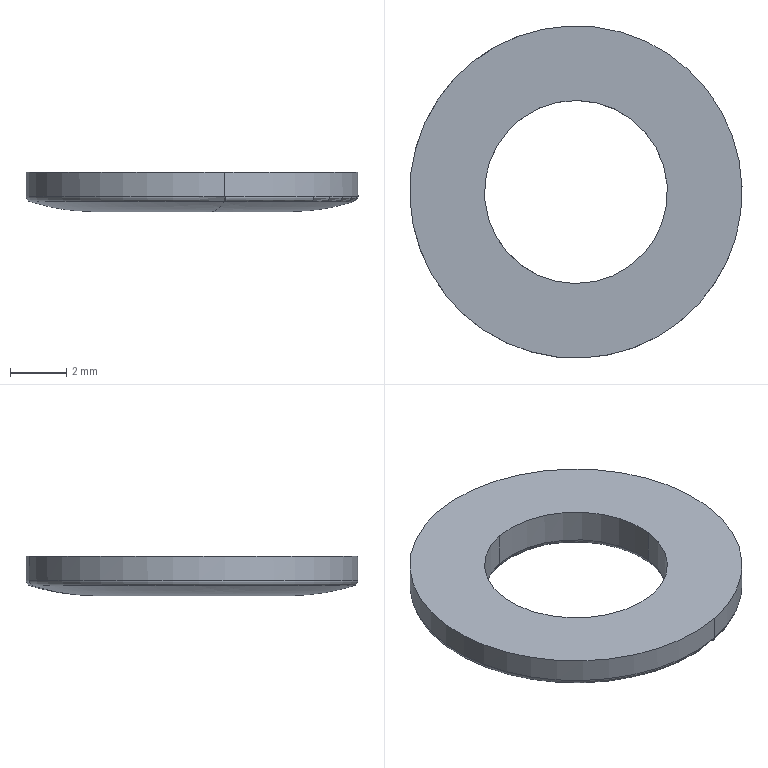Part | SolidWorks | features BaseBody 1 | 1 solid | 13 faces | box 11.8 x 11.8 x 1.4 mm | volume 95.374 mm3 | cylinder 6 | torus 4 | spline 2 | plane 1 | commonest cylinder face diameters 6.5 x3 11.8 x3
STEP:
#1=CARTESIAN_POINT('',(92.309,-207.694,-6.445));
#2=VERTEX_POINT('',#1);
#3=CARTESIAN_POINT('',(90.015,-196.407,-6.445));
#4=VERTEX_POINT('',#3);
#5=CARTESIAN_POINT('',(91.15,-202.053,-6.445));
#6=DIRECTION('',(0.,0.,1.));
#7=DIRECTION('',(0.2013,-0.9795,0.));
#8=AXIS2_PLACEMENT_3D('',#5,#6,#7);
#9=CIRCLE('',#8,5.759);
#10=EDGE_CURVE('',#2,#4,#9,.T.);
#11=ORIENTED_EDGE('',*,*,#10,.F.);
#12=CARTESIAN_POINT('',(92.284,-207.699,-6.445));
#13=VERTEX_POINT('',#12);
#14=CARTESIAN_POINT('',(91.15,-202.053,-6.445));
#15=DIRECTION('',(0.,0.,1.));
#16=DIRECTION('',(0.197,-0.9804,0.));
#17=AXIS2_PLACEMENT_3D('',#14,#15,#16);
#18=CIRCLE('',#17,5.759);
#19=EDGE_CURVE('',#13,#2,#18,.T.);
#20=ORIENTED_EDGE('',*,*,#19,.F.);
#21=CARTESIAN_POINT('',(91.83,-205.436,-6.8));
#22=VERTEX_POINT('',#21);
#23=CARTESIAN_POINT('',(91.82,-205.386,1.212));
#24=DIRECTION('',(-0.9804,-0.197,0.));
#25=DIRECTION('',(0.00126,-0.006272,-1.));
#26=AXIS2_PLACEMENT_3D('',#23,#24,#25);
#27=CIRCLE('',#26,8.012);
#28=EDGE_CURVE('',#22,#13,#27,.T.);
#29=ORIENTED_EDGE('',*,*,#28,.F.);
#30=CARTESIAN_POINT('',(90.488,-198.666,-6.8));
#31=VERTEX_POINT('',#30);
#32=CARTESIAN_POINT('',(91.15,-202.053,-6.8));
#33=DIRECTION('',(0.,0.,-1.));
#34=DIRECTION('',(-0.1918,0.9814,0.));
#35=AXIS2_PLACEMENT_3D('',#32,#33,#34);
#36=CIRCLE('',#35,3.451);
#37=EDGE_CURVE('',#31,#22,#36,.T.);
#38=ORIENTED_EDGE('',*,*,#37,.F.);
#39=CARTESIAN_POINT('',(90.47,-198.669,-6.8));
#40=VERTEX_POINT('',#39);
#41=CARTESIAN_POINT('',(91.15,-202.053,-6.8));
#42=DIRECTION('',(0.,0.,-1.));
#43=DIRECTION('',(-0.197,0.9804,0.));
#44=AXIS2_PLACEMENT_3D('',#41,#42,#43);
#45=CIRCLE('',#44,3.451);
#46=EDGE_CURVE('',#40,#31,#45,.T.);
#47=ORIENTED_EDGE('',*,*,#46,.F.);
#48=CARTESIAN_POINT('',(90.48,-198.719,1.212));
#49=DIRECTION('',(-0.9804,-0.197,0.));
#50=DIRECTION('',(-0.058,0.2886,-0.9557));
#51=AXIS2_PLACEMENT_3D('',#48,#49,#50);
#52=CIRCLE('',#51,8.012);
#53=EDGE_CURVE('',#4,#40,#52,.T.);
#54=ORIENTED_EDGE('',*,*,#53,.F.);
#55=EDGE_LOOP('',(#11,#20,#29,#38,#47,#54));
#56=FACE_OUTER_BOUND('',#55,.T.);
#57=CARTESIAN_POINT('',(91.6,-205.354,-6.8));
#58=CARTESIAN_POINT('',(91.716,-206.21,-6.807));
#59=CARTESIAN_POINT('',(91.832,-207.057,-6.676));
#60=CARTESIAN_POINT('',(91.943,-207.872,-6.409));
#61=CARTESIAN_POINT('',(93.631,-205.077,-6.8));
#62=CARTESIAN_POINT('',(94.275,-205.862,-6.807));
#63=CARTESIAN_POINT('',(94.912,-206.637,-6.676));
#64=CARTESIAN_POINT('',(95.524,-207.384,-6.409));
#65=CARTESIAN_POINT('',(94.819,-203.406,-6.8));
#66=CARTESIAN_POINT('',(95.772,-203.758,-6.807));
#67=CARTESIAN_POINT('',(96.714,-204.105,-6.676));
#68=CARTESIAN_POINT('',(97.62,-204.439,-6.409));
#69=CARTESIAN_POINT('',(94.416,-201.396,-6.8));
#70=CARTESIAN_POINT('',(95.263,-201.226,-6.807));
#71=CARTESIAN_POINT('',(96.101,-201.058,-6.676));
#72=CARTESIAN_POINT('',(96.908,-200.896,-6.409));
#73=CARTESIAN_POINT('',(94.012,-199.387,-6.8));
#74=CARTESIAN_POINT('',(94.755,-198.694,-6.807));
#75=CARTESIAN_POINT('',(95.489,-198.01,-6.676));
#76=CARTESIAN_POINT('',(96.196,-197.352,-6.409));
#77=CARTESIAN_POINT('',(92.27,-198.305,-6.8));
#78=CARTESIAN_POINT('',(92.561,-197.332,-6.807));
#79=CARTESIAN_POINT('',(92.848,-196.371,-6.676));
#80=CARTESIAN_POINT('',(93.125,-195.445,-6.409));
#81=CARTESIAN_POINT('',(90.29,-198.835,-6.8));
#82=CARTESIAN_POINT('',(90.066,-197.999,-6.807));
#83=CARTESIAN_POINT('',(89.846,-197.173,-6.676));
#84=CARTESIAN_POINT('',(89.633,-196.379,-6.409));
#85=(BOUNDED_SURFACE()B_SPLINE_SURFACE(3,3,((#57,#58,#59,#60),(#61,#62,#63,#64),(#65,#66,#67,#68),(#69,#70,#71,#72),(#73,#74,#75,#76),(#77,#78,#79,#80),(#81,#82,#83,#84)),.UNSPECIFIED.,.F.,.F.,.F.)B_SPLINE_SURFACE_WITH_KNOTS((4,3,4),(4,4),(0.,1.,2.),(0.,1.),.UNSPECIFIED.)GEOMETRIC_REPRESENTATION_ITEM()RATIONAL_B_SPLINE_SURFACE(((1.195,1.185,1.185,1.195),(0.9437,0.9355,0.9355,0.9437),(0.9437,0.9355,0.9355,0.9437),(1.195,1.185,1.185,1.195),(0.9437,0.9355,0.9355,0.9437),(0.9437,0.9355,0.9355,0.9437),(1.195,1.185,1.185,1.195)))REPRESENTATION_ITEM('')SURFACE());
#86=ADVANCED_FACE('',(#56),#85,.T.);
#87=CARTESIAN_POINT('',(89.99,-196.412,-6.445));
#88=VERTEX_POINT('',#87);
#89=CARTESIAN_POINT('',(91.15,-202.053,-6.445));
#90=DIRECTION('',(0.,0.,1.));
#91=DIRECTION('',(-0.2013,0.9795,0.));
#92=AXIS2_PLACEMENT_3D('',#89,#90,#91);
#93=CIRCLE('',#92,5.759);
#94=EDGE_CURVE('',#88,#13,#93,.T.);
#95=ORIENTED_EDGE('',*,*,#94,.F.);
#96=CARTESIAN_POINT('',(91.15,-202.053,-6.445));
#97=DIRECTION('',(0.,0.,1.));
#98=DIRECTION('',(-0.197,0.9804,0.));
#99=AXIS2_PLACEMENT_3D('',#96,#97,#98);
#100=CIRCLE('',#99,5.759);
#101=EDGE_CURVE('',#4,#88,#100,.T.);
#102=ORIENTED_EDGE('',*,*,#101,.F.);
#103=ORIENTED_EDGE('',*,*,#53,.T.);
#104=CARTESIAN_POINT('',(91.812,-205.44,-6.8));
#105=VERTEX_POINT('',#104);
#106=CARTESIAN_POINT('',(91.15,-202.053,-6.8));
#107=DIRECTION('',(0.,0.,-1.));
#108=DIRECTION('',(0.1918,-0.9814,0.));
#109=AXIS2_PLACEMENT_3D('',#106,#107,#108);
#110=CIRCLE('',#109,3.451);
#111=EDGE_CURVE('',#105,#40,#110,.T.);
#112=ORIENTED_EDGE('',*,*,#111,.F.);
#113=CARTESIAN_POINT('',(91.15,-202.053,-6.8));
#114=DIRECTION('',(0.,0.,-1.));
#115=DIRECTION('',(0.197,-0.9804,0.));
#116=AXIS2_PLACEMENT_3D('',#113,#114,#115);
#117=CIRCLE('',#116,3.451);
#118=EDGE_CURVE('',#22,#105,#117,.T.);
#119=ORIENTED_EDGE('',*,*,#118,.F.);
#120=ORIENTED_EDGE('',*,*,#28,.T.);
#121=EDGE_LOOP('',(#95,#102,#103,#112,#119,#120));
#122=FACE_OUTER_BOUND('',#121,.T.);
#123=CARTESIAN_POINT('',(90.7,-198.752,-6.8));
#124=CARTESIAN_POINT('',(90.583,-197.895,-6.807));
#125=CARTESIAN_POINT('',(90.467,-197.048,-6.676));
#126=CARTESIAN_POINT('',(90.356,-196.233,-6.409));
#127=CARTESIAN_POINT('',(88.668,-199.029,-6.8));
#128=CARTESIAN_POINT('',(88.024,-198.244,-6.807));
#129=CARTESIAN_POINT('',(87.388,-197.468,-6.676));
#130=CARTESIAN_POINT('',(86.775,-196.722,-6.409));
#131=CARTESIAN_POINT('',(87.48,-200.699,-6.8));
#132=CARTESIAN_POINT('',(86.527,-200.348,-6.807));
#133=CARTESIAN_POINT('',(85.585,-200.001,-6.676));
#134=CARTESIAN_POINT('',(84.679,-199.666,-6.409));
#135=CARTESIAN_POINT('',(87.884,-202.709,-6.8));
#136=CARTESIAN_POINT('',(87.036,-202.88,-6.807));
#137=CARTESIAN_POINT('',(86.198,-203.048,-6.676));
#138=CARTESIAN_POINT('',(85.391,-203.21,-6.409));
#139=CARTESIAN_POINT('',(88.288,-204.719,-6.8));
#140=CARTESIAN_POINT('',(87.545,-205.411,-6.807));
#141=CARTESIAN_POINT('',(86.81,-206.095,-6.676));
#142=CARTESIAN_POINT('',(86.104,-206.754,-6.409));
#143=CARTESIAN_POINT('',(90.029,-205.8,-6.8));
#144=CARTESIAN_POINT('',(89.738,-206.773,-6.807));
#145=CARTESIAN_POINT('',(89.451,-207.735,-6.676));
#146=CARTESIAN_POINT('',(89.174,-208.66,-6.409));
#147=CARTESIAN_POINT('',(92.01,-205.271,-6.8));
#148=CARTESIAN_POINT('',(92.233,-206.107,-6.807));
#149=CARTESIAN_POINT('',(92.454,-206.932,-6.676));
#150=CARTESIAN_POINT('',(92.666,-207.727,-6.409));
#151=(BOUNDED_SURFACE()B_SPLINE_SURFACE(3,3,((#123,#124,#125,#126),(#127,#128,#129,#130),(#131,#132,#133,#134),(#135,#136,#137,#138),(#139,#140,#141,#142),(#143,#144,#145,#146),(#147,#148,#149,#150)),.UNSPECIFIED.,.F.,.F.,.F.)B_SPLINE_SURFACE_WITH_KNOTS((4,3,4),(4,4),(0.,1.,2.),(0.,1.),.UNSPECIFIED.)GEOMETRIC_REPRESENTATION_ITEM()RATIONAL_B_SPLINE_SURFACE(((1.195,1.185,1.185,1.195),(0.9437,0.9355,0.9355,0.9437),(0.9437,0.9355,0.9355,0.9437),(1.195,1.185,1.185,1.195),(0.9437,0.9355,0.9355,0.9437),(0.9437,0.9355,0.9355,0.9437),(1.195,1.185,1.185,1.195)))REPRESENTATION_ITEM('')SURFACE());
#152=ADVANCED_FACE('',(#122),#151,.T.);
#153=ORIENTED_EDGE('',*,*,#37,.T.);
#154=ORIENTED_EDGE('',*,*,#118,.T.);
#155=CARTESIAN_POINT('',(91.773,-205.242,-6.6));
#156=VERTEX_POINT('',#155);
#157=CARTESIAN_POINT('',(91.811,-205.439,-6.6));
#158=DIRECTION('',(-0.9814,-0.1918,0.));
#159=DIRECTION('',(-0.1918,0.9814,0.));
#160=AXIS2_PLACEMENT_3D('',#157,#158,#159);
#161=CIRCLE('',#160,0.2);
#162=EDGE_CURVE('',#156,#105,#161,.T.);
#163=ORIENTED_EDGE('',*,*,#162,.F.);
#164=CARTESIAN_POINT('',(91.79,-205.239,-6.6));
#165=VERTEX_POINT('',#164);
#166=CARTESIAN_POINT('',(91.15,-202.053,-6.6));
#167=DIRECTION('',(0.,0.,-1.));
#168=DIRECTION('',(0.197,-0.9804,0.));
#169=AXIS2_PLACEMENT_3D('',#166,#167,#168);
#170=CIRCLE('',#169,3.25);
#171=EDGE_CURVE('',#165,#156,#170,.T.);
#172=ORIENTED_EDGE('',*,*,#171,.F.);
#173=CARTESIAN_POINT('',(94.374,-202.46,-6.6));
#174=VERTEX_POINT('',#173);
#175=CARTESIAN_POINT('',(91.15,-202.053,-6.6));
#176=DIRECTION('',(0.,0.,-1.));
#177=DIRECTION('',(0.9921,-0.1253,0.));
#178=AXIS2_PLACEMENT_3D('',#175,#176,#177);
#179=CIRCLE('',#178,3.25);
#180=EDGE_CURVE('',#174,#165,#179,.T.);
#181=ORIENTED_EDGE('',*,*,#180,.F.);
#182=CARTESIAN_POINT('',(90.526,-198.863,-6.6));
#183=VERTEX_POINT('',#182);
#184=CARTESIAN_POINT('',(91.15,-202.053,-6.6));
#185=DIRECTION('',(0.,0.,-1.));
#186=DIRECTION('',(0.9921,-0.1253,0.));
#187=AXIS2_PLACEMENT_3D('',#184,#185,#186);
#188=CIRCLE('',#187,3.25);
#189=EDGE_CURVE('',#183,#174,#188,.T.);
#190=ORIENTED_EDGE('',*,*,#189,.F.);
#191=CARTESIAN_POINT('',(90.488,-198.667,-6.6));
#192=DIRECTION('',(-0.9814,-0.1918,0.));
#193=DIRECTION('',(-0.001205,0.006167,-1.));
#194=AXIS2_PLACEMENT_3D('',#191,#192,#193);
#195=CIRCLE('',#194,0.2);
#196=EDGE_CURVE('',#31,#183,#195,.T.);
#197=ORIENTED_EDGE('',*,*,#196,.F.);
#198=EDGE_LOOP('',(#153,#154,#163,#172,#181,#190,#197));
#199=FACE_OUTER_BOUND('',#198,.T.);
#200=CARTESIAN_POINT('',(91.15,-202.053,-6.6));
#201=DIRECTION('',(0.,0.,-1.));
#202=DIRECTION('',(-0.1918,0.9814,0.));
#203=AXIS2_PLACEMENT_3D('',#200,#201,#202);
#204=TOROIDAL_SURFACE('',#203,3.45,0.2);
#205=ADVANCED_FACE('',(#199),#204,.T.);
#206=ORIENTED_EDGE('',*,*,#111,.T.);
#207=ORIENTED_EDGE('',*,*,#46,.T.);
#208=ORIENTED_EDGE('',*,*,#196,.T.);
#209=CARTESIAN_POINT('',(90.509,-198.867,-6.6));
#210=VERTEX_POINT('',#209);
#211=CARTESIAN_POINT('',(91.15,-202.053,-6.6));
#212=DIRECTION('',(0.,0.,-1.));
#213=DIRECTION('',(-0.197,0.9804,0.));
#214=AXIS2_PLACEMENT_3D('',#211,#212,#213);
#215=CIRCLE('',#214,3.25);
#216=EDGE_CURVE('',#210,#183,#215,.T.);
#217=ORIENTED_EDGE('',*,*,#216,.F.);
#218=CARTESIAN_POINT('',(91.15,-202.053,-6.6));
#219=DIRECTION('',(0.,0.,-1.));
#220=DIRECTION('',(-0.9921,0.1253,0.));
#221=AXIS2_PLACEMENT_3D('',#218,#219,#220);
#222=CIRCLE('',#221,3.25);
#223=EDGE_CURVE('',#156,#210,#222,.T.);
#224=ORIENTED_EDGE('',*,*,#223,.F.);
#225=ORIENTED_EDGE('',*,*,#162,.T.);
#226=EDGE_LOOP('',(#206,#207,#208,#217,#224,#225));
#227=FACE_OUTER_BOUND('',#226,.T.);
#228=CARTESIAN_POINT('',(91.15,-202.053,-6.6));
#229=DIRECTION('',(0.,0.,-1.));
#230=DIRECTION('',(0.1918,-0.9814,0.));
#231=AXIS2_PLACEMENT_3D('',#228,#229,#230);
#232=TOROIDAL_SURFACE('',#231,3.45,0.2);
#233=ADVANCED_FACE('',(#227),#232,.T.);
#234=ORIENTED_EDGE('',*,*,#171,.T.);
#235=ORIENTED_EDGE('',*,*,#223,.T.);
#236=CARTESIAN_POINT('',(90.509,-198.867,-5.4));
#237=VERTEX_POINT('',#236);
#238=CARTESIAN_POINT('',(90.509,-198.867,-6.6));
#239=DIRECTION('',(0.,0.,1.));
#240=VECTOR('',#239,1000.);
#241=LINE('',#238,#240);
#242=EDGE_CURVE('',#210,#237,#241,.T.);
#243=ORIENTED_EDGE('',*,*,#242,.T.);
#244=CARTESIAN_POINT('',(91.79,-205.239,-5.4));
#245=VERTEX_POINT('',#244);
#246=CARTESIAN_POINT('',(91.15,-202.053,-5.4));
#247=DIRECTION('',(0.,0.,1.));
#248=DIRECTION('',(-0.197,0.9804,0.));
#249=AXIS2_PLACEMENT_3D('',#246,#247,#248);
#250=CIRCLE('',#249,3.25);
#251=EDGE_CURVE('',#237,#245,#250,.T.);
#252=ORIENTED_EDGE('',*,*,#251,.T.);
#253=CARTESIAN_POINT('',(91.79,-205.239,-5.4));
#254=DIRECTION('',(0.,0.,-1.));
#255=VECTOR('',#254,1000.);
#256=LINE('',#253,#255);
#257=EDGE_CURVE('',#245,#165,#256,.T.);
#258=ORIENTED_EDGE('',*,*,#257,.T.);
#259=EDGE_LOOP('',(#234,#235,#243,#252,#258));
#260=FACE_OUTER_BOUND('',#259,.T.);
#261=CARTESIAN_POINT('',(91.15,-202.053,-6.));
#262=DIRECTION('',(0.,0.,-1.));
#263=DIRECTION('',(0.9921,-0.1253,0.));
#264=AXIS2_PLACEMENT_3D('',#261,#262,#263);
#265=CYLINDRICAL_SURFACE('',#264,3.25);
#266=ADVANCED_FACE('',(#260),#265,.F.);
#267=CARTESIAN_POINT('',(94.374,-202.46,-5.4));
#268=VERTEX_POINT('',#267);
#269=CARTESIAN_POINT('',(94.374,-202.46,-6.));
#270=DIRECTION('',(0.,0.,-1.));
#271=VECTOR('',#270,1000.);
#272=LINE('',#269,#271);
#273=EDGE_CURVE('',#268,#174,#272,.T.);
#274=ORIENTED_EDGE('',*,*,#273,.F.);
#275=CARTESIAN_POINT('',(91.15,-202.053,-5.4));
#276=DIRECTION('',(0.,0.,1.));
#277=DIRECTION('',(0.9921,-0.1253,0.));
#278=AXIS2_PLACEMENT_3D('',#275,#276,#277);
#279=CIRCLE('',#278,3.25);
#280=EDGE_CURVE('',#268,#237,#279,.T.);
#281=ORIENTED_EDGE('',*,*,#280,.T.);
#282=ORIENTED_EDGE('',*,*,#242,.F.);
#283=ORIENTED_EDGE('',*,*,#216,.T.);
#284=ORIENTED_EDGE('',*,*,#189,.T.);
#285=EDGE_LOOP('',(#274,#281,#282,#283,#284));
#286=FACE_OUTER_BOUND('',#285,.T.);
#287=CARTESIAN_POINT('',(91.15,-202.053,-6.));
#288=DIRECTION('',(0.,0.,-1.));
#289=DIRECTION('',(0.9921,-0.1253,0.));
#290=AXIS2_PLACEMENT_3D('',#287,#288,#289);
#291=CYLINDRICAL_SURFACE('',#290,3.25);
#292=ADVANCED_FACE('',(#286),#291,.F.);
#293=CARTESIAN_POINT('',(91.15,-202.053,-5.4));
#294=DIRECTION('',(0.,0.,1.));
#295=DIRECTION('',(0.9921,-0.1253,0.));
#296=AXIS2_PLACEMENT_3D('',#293,#294,#295);
#297=CIRCLE('',#296,3.25);
#298=EDGE_CURVE('',#245,#268,#297,.T.);
#299=ORIENTED_EDGE('',*,*,#298,.F.);
#300=ORIENTED_EDGE('',*,*,#251,.F.);
#301=ORIENTED_EDGE('',*,*,#280,.F.);
#302=EDGE_LOOP('',(#299,#300,#301));
#303=FACE_BOUND('',#302,.T.);
#304=CARTESIAN_POINT('',(89.987,-196.268,-5.4));
#305=VERTEX_POINT('',#304);
#306=CARTESIAN_POINT('',(97.003,-202.792,-5.4));
#307=VERTEX_POINT('',#306);
#308=CARTESIAN_POINT('',(91.15,-202.053,-5.4));
#309=DIRECTION('',(0.,0.,-1.));
#310=DIRECTION('',(-0.197,0.9804,0.));
#311=AXIS2_PLACEMENT_3D('',#308,#309,#310);
#312=CIRCLE('',#311,5.9);
#313=EDGE_CURVE('',#305,#307,#312,.T.);
#314=ORIENTED_EDGE('',*,*,#313,.F.);
#315=CARTESIAN_POINT('',(92.312,-207.837,-5.4));
#316=VERTEX_POINT('',#315);
#317=CARTESIAN_POINT('',(91.15,-202.053,-5.4));
#318=DIRECTION('',(0.,0.,-1.));
#319=DIRECTION('',(-0.9921,0.1253,0.));
#320=AXIS2_PLACEMENT_3D('',#317,#318,#319);
#321=CIRCLE('',#320,5.9);
#322=EDGE_CURVE('',#316,#305,#321,.T.);
#323=ORIENTED_EDGE('',*,*,#322,.F.);
#324=CARTESIAN_POINT('',(91.15,-202.053,-5.4));
#325=DIRECTION('',(0.,0.,-1.));
#326=DIRECTION('',(-0.197,0.9804,0.));
#327=AXIS2_PLACEMENT_3D('',#324,#325,#326);
#328=CIRCLE('',#327,5.9);
#329=EDGE_CURVE('',#307,#316,#328,.T.);
#330=ORIENTED_EDGE('',*,*,#329,.F.);
#331=EDGE_LOOP('',(#314,#323,#330));
#332=FACE_OUTER_BOUND('',#331,.T.);
#333=CARTESIAN_POINT('',(85.603,-210.389,-5.4));
#334=DIRECTION('',(0.,0.,1.));
#335=DIRECTION('',(1.,0.,0.));
#336=AXIS2_PLACEMENT_3D('',#333,#334,#335);
#337=PLANE('',#336);
#338=ADVANCED_FACE('',(#303,#332),#337,.T.);
#339=CARTESIAN_POINT('',(97.003,-202.792,-6.254));
#340=VERTEX_POINT('',#339);
#341=CARTESIAN_POINT('',(97.003,-202.792,-5.827));
#342=DIRECTION('',(0.,0.,-1.));
#343=VECTOR('',#342,1000.);
#344=LINE('',#341,#343);
#345=EDGE_CURVE('',#307,#340,#344,.T.);
#346=ORIENTED_EDGE('',*,*,#345,.F.);
#347=ORIENTED_EDGE('',*,*,#329,.T.);
#348=CARTESIAN_POINT('',(92.312,-207.837,-6.254));
#349=VERTEX_POINT('',#348);
#350=CARTESIAN_POINT('',(92.312,-207.837,-6.254));
#351=DIRECTION('',(0.,0.,1.));
#352=VECTOR('',#351,1000.);
#353=LINE('',#350,#352);
#354=EDGE_CURVE('',#349,#316,#353,.T.);
#355=ORIENTED_EDGE('',*,*,#354,.F.);
#356=CARTESIAN_POINT('',(92.337,-207.832,-6.254));
#357=VERTEX_POINT('',#356);
#358=CARTESIAN_POINT('',(91.15,-202.053,-6.254));
#359=DIRECTION('',(0.,0.,1.));
#360=DIRECTION('',(0.197,-0.9804,0.));
#361=AXIS2_PLACEMENT_3D('',#358,#359,#360);
#362=CIRCLE('',#361,5.9);
#363=EDGE_CURVE('',#349,#357,#362,.T.);
#364=ORIENTED_EDGE('',*,*,#363,.T.);
#365=CARTESIAN_POINT('',(91.15,-202.053,-6.254));
#366=DIRECTION('',(0.,0.,1.));
#367=DIRECTION('',(0.2013,-0.9795,0.));
#368=AXIS2_PLACEMENT_3D('',#365,#366,#367);
#369=CIRCLE('',#368,5.9);
#370=EDGE_CURVE('',#357,#340,#369,.T.);
#371=ORIENTED_EDGE('',*,*,#370,.T.);
#372=EDGE_LOOP('',(#346,#347,#355,#364,#371));
#373=FACE_OUTER_BOUND('',#372,.T.);
#374=CARTESIAN_POINT('',(91.15,-202.053,-5.827));
#375=DIRECTION('',(0.,0.,-1.));
#376=DIRECTION('',(0.9921,-0.1253,0.));
#377=AXIS2_PLACEMENT_3D('',#374,#375,#376);
#378=CYLINDRICAL_SURFACE('',#377,5.9);
#379=ADVANCED_FACE('',(#373),#378,.T.);
#380=ORIENTED_EDGE('',*,*,#354,.T.);
#381=ORIENTED_EDGE('',*,*,#322,.T.);
#382=CARTESIAN_POINT('',(89.987,-196.268,-6.254));
#383=VERTEX_POINT('',#382);
#384=CARTESIAN_POINT('',(89.987,-196.268,-5.4));
#385=DIRECTION('',(0.,0.,-1.));
#386=VECTOR('',#385,1000.);
#387=LINE('',#384,#386);
#388=EDGE_CURVE('',#305,#383,#387,.T.);
#389=ORIENTED_EDGE('',*,*,#388,.T.);
#390=CARTESIAN_POINT('',(89.962,-196.274,-6.254));
#391=VERTEX_POINT('',#390);
#392=CARTESIAN_POINT('',(91.15,-202.053,-6.254));
#393=DIRECTION('',(0.,0.,1.));
#394=DIRECTION('',(-0.197,0.9804,0.));
#395=AXIS2_PLACEMENT_3D('',#392,#393,#394);
#396=CIRCLE('',#395,5.9);
#397=EDGE_CURVE('',#383,#391,#396,.T.);
#398=ORIENTED_EDGE('',*,*,#397,.T.);
#399=CARTESIAN_POINT('',(91.15,-202.053,-6.254));
#400=DIRECTION('',(0.,0.,1.));
#401=DIRECTION('',(-0.2013,0.9795,0.));
#402=AXIS2_PLACEMENT_3D('',#399,#400,#401);
#403=CIRCLE('',#402,5.9);
#404=EDGE_CURVE('',#391,#349,#403,.T.);
#405=ORIENTED_EDGE('',*,*,#404,.T.);
#406=EDGE_LOOP('',(#380,#381,#389,#398,#405));
#407=FACE_OUTER_BOUND('',#406,.T.);
#408=CARTESIAN_POINT('',(91.15,-202.053,-5.827));
#409=DIRECTION('',(0.,0.,-1.));
#410=DIRECTION('',(0.9921,-0.1253,0.));
#411=AXIS2_PLACEMENT_3D('',#408,#409,#410);
#412=CYLINDRICAL_SURFACE('',#411,5.9);
#413=ADVANCED_FACE('',(#407),#412,.T.);
#414=ORIENTED_EDGE('',*,*,#363,.F.);
#415=ORIENTED_EDGE('',*,*,#404,.F.);
#416=CARTESIAN_POINT('',(90.002,-196.469,-6.254));
#417=DIRECTION('',(-0.9795,-0.2013,0.));
#418=DIRECTION('',(-0.2013,0.9795,0.));
#419=AXIS2_PLACEMENT_3D('',#416,#417,#418);
#420=CIRCLE('',#419,0.2);
#421=EDGE_CURVE('',#391,#88,#420,.T.);
#422=ORIENTED_EDGE('',*,*,#421,.T.);
#423=ORIENTED_EDGE('',*,*,#94,.T.);
#424=ORIENTED_EDGE('',*,*,#19,.T.);
#425=CARTESIAN_POINT('',(92.297,-207.636,-6.254));
#426=DIRECTION('',(-0.9795,-0.2013,0.));
#427=DIRECTION('',(0.05923,-0.2882,-0.9557));
#428=AXIS2_PLACEMENT_3D('',#425,#426,#427);
#429=CIRCLE('',#428,0.2);
#430=EDGE_CURVE('',#2,#357,#429,.T.);
#431=ORIENTED_EDGE('',*,*,#430,.T.);
#432=EDGE_LOOP('',(#414,#415,#422,#423,#424,#431));
#433=FACE_OUTER_BOUND('',#432,.T.);
#434=CARTESIAN_POINT('',(91.15,-202.053,-6.254));
#435=DIRECTION('',(0.,0.,1.));
#436=DIRECTION('',(0.2013,-0.9795,0.));
#437=AXIS2_PLACEMENT_3D('',#434,#435,#436);
#438=TOROIDAL_SURFACE('',#437,5.7,0.2);
#439=ADVANCED_FACE('',(#433),#438,.T.);
#440=ORIENTED_EDGE('',*,*,#397,.F.);
#441=CARTESIAN_POINT('',(91.15,-202.053,-6.254));
#442=DIRECTION('',(0.,0.,1.));
#443=DIRECTION('',(0.2013,-0.9795,0.));
#444=AXIS2_PLACEMENT_3D('',#441,#442,#443);
#445=CIRCLE('',#444,5.9);
#446=EDGE_CURVE('',#340,#383,#445,.T.);
#447=ORIENTED_EDGE('',*,*,#446,.F.);
#448=ORIENTED_EDGE('',*,*,#370,.F.);
#449=ORIENTED_EDGE('',*,*,#430,.F.);
#450=ORIENTED_EDGE('',*,*,#10,.T.);
#451=ORIENTED_EDGE('',*,*,#101,.T.);
#452=ORIENTED_EDGE('',*,*,#421,.F.);
#453=EDGE_LOOP('',(#440,#447,#448,#449,#450,#451,#452));
#454=FACE_OUTER_BOUND('',#453,.T.);
#455=CARTESIAN_POINT('',(91.15,-202.053,-6.254));
#456=DIRECTION('',(0.,0.,1.));
#457=DIRECTION('',(-0.2013,0.9795,0.));
#458=AXIS2_PLACEMENT_3D('',#455,#456,#457);
#459=TOROIDAL_SURFACE('',#458,5.7,0.2);
#460=ADVANCED_FACE('',(#454),#459,.T.);
#461=ORIENTED_EDGE('',*,*,#313,.T.);
#462=ORIENTED_EDGE('',*,*,#345,.T.);
#463=ORIENTED_EDGE('',*,*,#446,.T.);
#464=ORIENTED_EDGE('',*,*,#388,.F.);
#465=EDGE_LOOP('',(#461,#462,#463,#464));
#466=FACE_OUTER_BOUND('',#465,.T.);
#467=CARTESIAN_POINT('',(91.15,-202.053,-5.827));
#468=DIRECTION('',(0.,0.,-1.));
#469=DIRECTION('',(0.9921,-0.1253,0.));
#470=AXIS2_PLACEMENT_3D('',#467,#468,#469);
#471=CYLINDRICAL_SURFACE('',#470,5.9);
#472=ADVANCED_FACE('',(#466),#471,.T.);
#473=ORIENTED_EDGE('',*,*,#298,.T.);
#474=ORIENTED_EDGE('',*,*,#273,.T.);
#475=ORIENTED_EDGE('',*,*,#180,.T.);
#476=ORIENTED_EDGE('',*,*,#257,.F.);
#477=EDGE_LOOP('',(#473,#474,#475,#476));
#478=FACE_OUTER_BOUND('',#477,.T.);
#479=CARTESIAN_POINT('',(91.15,-202.053,-6.));
#480=DIRECTION('',(0.,0.,-1.));
#481=DIRECTION('',(0.9921,-0.1253,0.));
#482=AXIS2_PLACEMENT_3D('',#479,#480,#481);
#483=CYLINDRICAL_SURFACE('',#482,3.25);
#484=ADVANCED_FACE('',(#478),#483,.F.);
#485=CLOSED_SHELL('',(#86,#152,#205,#233,#266,#292,#338,#379,#413,#439,#460,#472,#484));
#486=MANIFOLD_SOLID_BREP('',#485);
#487=CARTESIAN_POINT('',(0.,0.,0.));
#488=DIRECTION('',(0.,0.,1.));
#489=DIRECTION('',(1.,0.,0.));
#490=AXIS2_PLACEMENT_3D('',#487,#488,#489);
#491=(LENGTH_UNIT()NAMED_UNIT(*)SI_UNIT(.MILLI.,.METRE.));
#492=UNCERTAINTY_MEASURE_WITH_UNIT(LENGTH_MEASURE(0.00001),#491,'','');
#493=(NAMED_UNIT(*)PLANE_ANGLE_UNIT()SI_UNIT($,.RADIAN.));
#494=(NAMED_UNIT(*)SI_UNIT($,.STERADIAN.)SOLID_ANGLE_UNIT());
#495=(GEOMETRIC_REPRESENTATION_CONTEXT(3)GLOBAL_UNCERTAINTY_ASSIGNED_CONTEXT((#492))GLOBAL_UNIT_ASSIGNED_CONTEXT((#491,#493,#494))REPRESENTATION_CONTEXT('',''));
#496=ADVANCED_BREP_SHAPE_REPRESENTATION('',(#486,#490),#495);